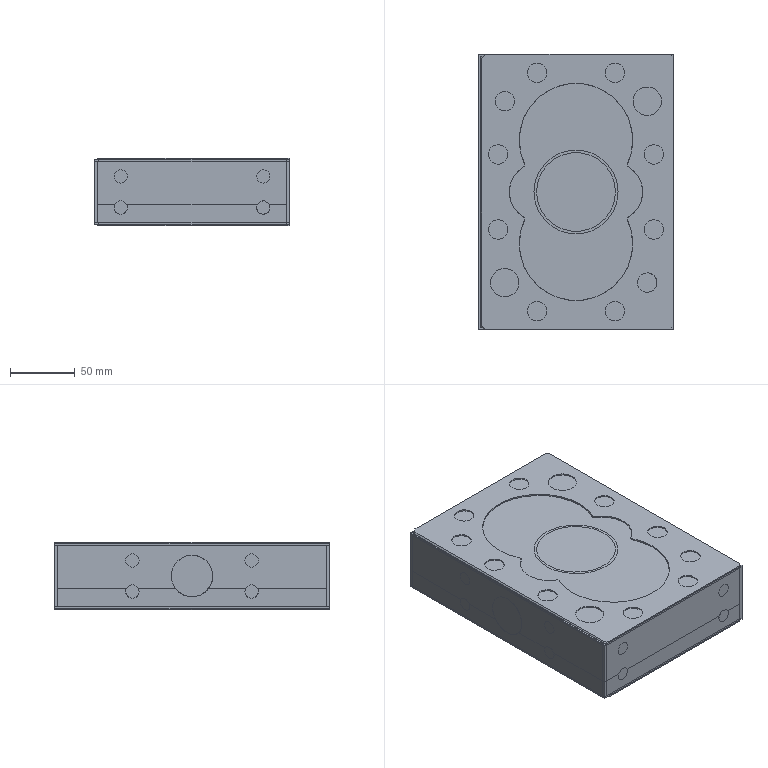Part | 6 solids | 250 faces | box 150.2 x 212.2 x 52.4 mm | volume 3895887 mm3 | plane 127 | cylinder 123 | commonest cylinder face diameters 10.2 x42 15 x40 32 x8 20.5 x6 22 x6 45 x4